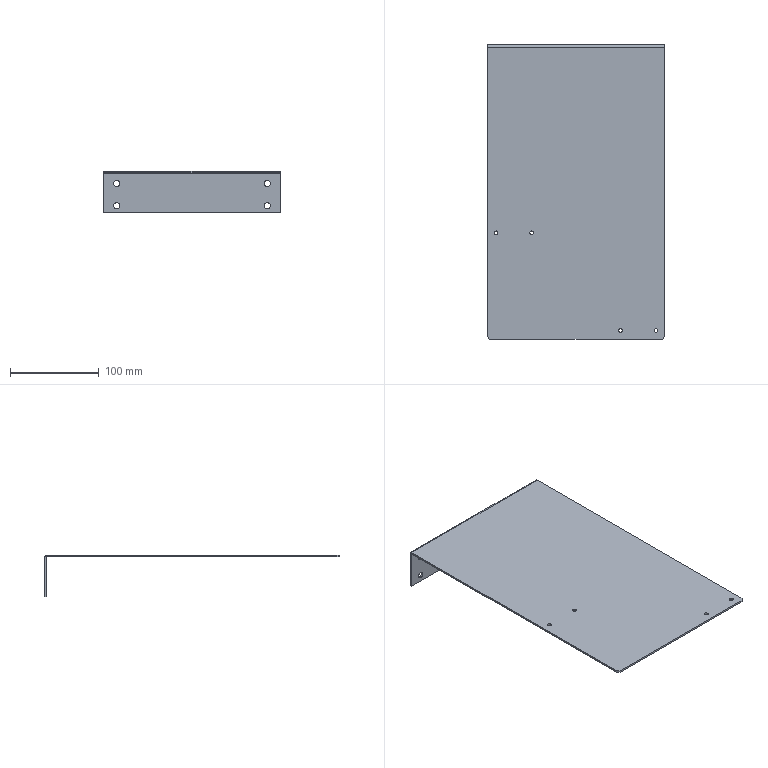Part | SolidWorks | features BaseBody 1 | 1 solid | 28 faces | box 200 x 332 x 47 mm | volume 150065 mm3 | cylinder 18 | plane 10 | commonest cylinder face diameters 4.2 x8 7 x8 1.473 x1 5.473 x1
STEP:
#1=CARTESIAN_POINT('',(85.,0.,-15.5));
#2=VERTEX_POINT('',#1);
#3=CARTESIAN_POINT('',(85.,0.,-8.5));
#4=VERTEX_POINT('',#3);
#5=CARTESIAN_POINT('',(85.,0.,-12.));
#6=DIRECTION('',(0.,1.,0.));
#7=DIRECTION('',(0.,0.,-1.));
#8=AXIS2_PLACEMENT_3D('',#5,#6,#7);
#9=CIRCLE('',#8,3.5);
#10=EDGE_CURVE('',#2,#4,#9,.T.);
#11=ORIENTED_EDGE('',*,*,#10,.F.);
#12=CARTESIAN_POINT('',(85.,2.,-15.5));
#13=VERTEX_POINT('',#12);
#14=CARTESIAN_POINT('',(85.,-330.001,-15.5));
#15=DIRECTION('',(0.,1.,0.));
#16=VECTOR('',#15,1000.);
#17=LINE('',#14,#16);
#18=EDGE_CURVE('',#2,#13,#17,.T.);
#19=ORIENTED_EDGE('',*,*,#18,.T.);
#20=CARTESIAN_POINT('',(85.,2.,-8.5));
#21=VERTEX_POINT('',#20);
#22=CARTESIAN_POINT('',(85.,2.,-12.));
#23=DIRECTION('',(0.,1.,0.));
#24=DIRECTION('',(0.,0.,1.));
#25=AXIS2_PLACEMENT_3D('',#22,#23,#24);
#26=CIRCLE('',#25,3.5);
#27=EDGE_CURVE('',#13,#21,#26,.T.);
#28=ORIENTED_EDGE('',*,*,#27,.T.);
#29=CARTESIAN_POINT('',(85.,-330.001,-8.5));
#30=DIRECTION('',(0.,1.,0.));
#31=VECTOR('',#30,1000.);
#32=LINE('',#29,#31);
#33=EDGE_CURVE('',#4,#21,#32,.T.);
#34=ORIENTED_EDGE('',*,*,#33,.F.);
#35=EDGE_LOOP('',(#11,#19,#28,#34));
#36=FACE_OUTER_BOUND('',#35,.T.);
#37=CARTESIAN_POINT('',(85.,-330.001,-12.));
#38=DIRECTION('',(0.,1.,0.));
#39=DIRECTION('',(0.,0.,1.));
#40=AXIS2_PLACEMENT_3D('',#37,#38,#39);
#41=CYLINDRICAL_SURFACE('',#40,3.5);
#42=ADVANCED_FACE('',(#36),#41,.F.);
#43=CARTESIAN_POINT('',(85.,0.,-40.5));
#44=VERTEX_POINT('',#43);
#45=CARTESIAN_POINT('',(85.,0.,-33.5));
#46=VERTEX_POINT('',#45);
#47=CARTESIAN_POINT('',(85.,0.,-37.));
#48=DIRECTION('',(0.,1.,0.));
#49=DIRECTION('',(0.,0.,-1.));
#50=AXIS2_PLACEMENT_3D('',#47,#48,#49);
#51=CIRCLE('',#50,3.5);
#52=EDGE_CURVE('',#44,#46,#51,.T.);
#53=ORIENTED_EDGE('',*,*,#52,.F.);
#54=CARTESIAN_POINT('',(85.,2.,-40.5));
#55=VERTEX_POINT('',#54);
#56=CARTESIAN_POINT('',(85.,-330.001,-40.5));
#57=DIRECTION('',(0.,1.,0.));
#58=VECTOR('',#57,1000.);
#59=LINE('',#56,#58);
#60=EDGE_CURVE('',#44,#55,#59,.T.);
#61=ORIENTED_EDGE('',*,*,#60,.T.);
#62=CARTESIAN_POINT('',(85.,2.,-33.5));
#63=VERTEX_POINT('',#62);
#64=CARTESIAN_POINT('',(85.,2.,-37.));
#65=DIRECTION('',(0.,1.,0.));
#66=DIRECTION('',(0.,0.,-1.));
#67=AXIS2_PLACEMENT_3D('',#64,#65,#66);
#68=CIRCLE('',#67,3.5);
#69=EDGE_CURVE('',#55,#63,#68,.T.);
#70=ORIENTED_EDGE('',*,*,#69,.T.);
#71=CARTESIAN_POINT('',(85.,-330.001,-33.5));
#72=DIRECTION('',(0.,1.,0.));
#73=VECTOR('',#72,1000.);
#74=LINE('',#71,#73);
#75=EDGE_CURVE('',#46,#63,#74,.T.);
#76=ORIENTED_EDGE('',*,*,#75,.F.);
#77=EDGE_LOOP('',(#53,#61,#70,#76));
#78=FACE_OUTER_BOUND('',#77,.T.);
#79=CARTESIAN_POINT('',(85.,-330.001,-37.));
#80=DIRECTION('',(0.,1.,0.));
#81=DIRECTION('',(0.,0.,1.));
#82=AXIS2_PLACEMENT_3D('',#79,#80,#81);
#83=CYLINDRICAL_SURFACE('',#82,3.5);
#84=ADVANCED_FACE('',(#78),#83,.F.);
#85=CARTESIAN_POINT('',(-85.,0.,-15.5));
#86=VERTEX_POINT('',#85);
#87=CARTESIAN_POINT('',(-85.,0.,-8.5));
#88=VERTEX_POINT('',#87);
#89=CARTESIAN_POINT('',(-85.,0.,-12.));
#90=DIRECTION('',(0.,1.,0.));
#91=DIRECTION('',(0.,0.,-1.));
#92=AXIS2_PLACEMENT_3D('',#89,#90,#91);
#93=CIRCLE('',#92,3.5);
#94=EDGE_CURVE('',#86,#88,#93,.T.);
#95=ORIENTED_EDGE('',*,*,#94,.F.);
#96=CARTESIAN_POINT('',(-85.,2.,-15.5));
#97=VERTEX_POINT('',#96);
#98=CARTESIAN_POINT('',(-85.,-330.001,-15.5));
#99=DIRECTION('',(0.,1.,0.));
#100=VECTOR('',#99,1000.);
#101=LINE('',#98,#100);
#102=EDGE_CURVE('',#86,#97,#101,.T.);
#103=ORIENTED_EDGE('',*,*,#102,.T.);
#104=CARTESIAN_POINT('',(-85.,2.,-8.5));
#105=VERTEX_POINT('',#104);
#106=CARTESIAN_POINT('',(-85.,2.,-12.));
#107=DIRECTION('',(0.,1.,0.));
#108=DIRECTION('',(0.,0.,-1.));
#109=AXIS2_PLACEMENT_3D('',#106,#107,#108);
#110=CIRCLE('',#109,3.5);
#111=EDGE_CURVE('',#97,#105,#110,.T.);
#112=ORIENTED_EDGE('',*,*,#111,.T.);
#113=CARTESIAN_POINT('',(-85.,-330.001,-8.5));
#114=DIRECTION('',(0.,1.,0.));
#115=VECTOR('',#114,1000.);
#116=LINE('',#113,#115);
#117=EDGE_CURVE('',#88,#105,#116,.T.);
#118=ORIENTED_EDGE('',*,*,#117,.F.);
#119=EDGE_LOOP('',(#95,#103,#112,#118));
#120=FACE_OUTER_BOUND('',#119,.T.);
#121=CARTESIAN_POINT('',(-85.,-330.001,-12.));
#122=DIRECTION('',(0.,1.,0.));
#123=DIRECTION('',(0.,0.,1.));
#124=AXIS2_PLACEMENT_3D('',#121,#122,#123);
#125=CYLINDRICAL_SURFACE('',#124,3.5);
#126=ADVANCED_FACE('',(#120),#125,.F.);
#127=CARTESIAN_POINT('',(-85.,0.,-40.5));
#128=VERTEX_POINT('',#127);
#129=CARTESIAN_POINT('',(-85.,0.,-33.5));
#130=VERTEX_POINT('',#129);
#131=CARTESIAN_POINT('',(-85.,0.,-37.));
#132=DIRECTION('',(0.,1.,0.));
#133=DIRECTION('',(0.,0.,-1.));
#134=AXIS2_PLACEMENT_3D('',#131,#132,#133);
#135=CIRCLE('',#134,3.5);
#136=EDGE_CURVE('',#128,#130,#135,.T.);
#137=ORIENTED_EDGE('',*,*,#136,.F.);
#138=CARTESIAN_POINT('',(-85.,2.,-40.5));
#139=VERTEX_POINT('',#138);
#140=CARTESIAN_POINT('',(-85.,-330.001,-40.5));
#141=DIRECTION('',(0.,1.,0.));
#142=VECTOR('',#141,1000.);
#143=LINE('',#140,#142);
#144=EDGE_CURVE('',#128,#139,#143,.T.);
#145=ORIENTED_EDGE('',*,*,#144,.T.);
#146=CARTESIAN_POINT('',(-85.,2.,-33.5));
#147=VERTEX_POINT('',#146);
#148=CARTESIAN_POINT('',(-85.,2.,-37.));
#149=DIRECTION('',(0.,1.,0.));
#150=DIRECTION('',(0.,0.,1.));
#151=AXIS2_PLACEMENT_3D('',#148,#149,#150);
#152=CIRCLE('',#151,3.5);
#153=EDGE_CURVE('',#139,#147,#152,.T.);
#154=ORIENTED_EDGE('',*,*,#153,.T.);
#155=CARTESIAN_POINT('',(-85.,-330.001,-33.5));
#156=DIRECTION('',(0.,1.,0.));
#157=VECTOR('',#156,1000.);
#158=LINE('',#155,#157);
#159=EDGE_CURVE('',#130,#147,#158,.T.);
#160=ORIENTED_EDGE('',*,*,#159,.F.);
#161=EDGE_LOOP('',(#137,#145,#154,#160));
#162=FACE_OUTER_BOUND('',#161,.T.);
#163=CARTESIAN_POINT('',(-85.,-330.001,-37.));
#164=DIRECTION('',(0.,1.,0.));
#165=DIRECTION('',(0.,0.,1.));
#166=AXIS2_PLACEMENT_3D('',#163,#164,#165);
#167=CYLINDRICAL_SURFACE('',#166,3.5);
#168=ADVANCED_FACE('',(#162),#167,.F.);
#169=CARTESIAN_POINT('',(90.,-322.1,2.));
#170=VERTEX_POINT('',#169);
#171=CARTESIAN_POINT('',(90.,-317.9,2.));
#172=VERTEX_POINT('',#171);
#173=CARTESIAN_POINT('',(90.,-320.,2.));
#174=DIRECTION('',(0.,0.,-1.));
#175=DIRECTION('',(0.,1.,0.));
#176=AXIS2_PLACEMENT_3D('',#173,#174,#175);
#177=CIRCLE('',#176,2.1);
#178=EDGE_CURVE('',#170,#172,#177,.T.);
#179=ORIENTED_EDGE('',*,*,#178,.F.);
#180=CARTESIAN_POINT('',(90.,-322.1,0.));
#181=VERTEX_POINT('',#180);
#182=CARTESIAN_POINT('',(90.,-322.1,0.));
#183=DIRECTION('',(0.,0.,-1.));
#184=VECTOR('',#183,1000.);
#185=LINE('',#182,#184);
#186=EDGE_CURVE('',#170,#181,#185,.T.);
#187=ORIENTED_EDGE('',*,*,#186,.T.);
#188=CARTESIAN_POINT('',(90.,-317.9,0.));
#189=VERTEX_POINT('',#188);
#190=CARTESIAN_POINT('',(90.,-320.,0.));
#191=DIRECTION('',(0.,0.,-1.));
#192=DIRECTION('',(0.,1.,0.));
#193=AXIS2_PLACEMENT_3D('',#190,#191,#192);
#194=CIRCLE('',#193,2.1);
#195=EDGE_CURVE('',#181,#189,#194,.T.);
#196=ORIENTED_EDGE('',*,*,#195,.T.);
#197=CARTESIAN_POINT('',(90.,-317.9,0.));
#198=DIRECTION('',(0.,0.,-1.));
#199=VECTOR('',#198,1000.);
#200=LINE('',#197,#199);
#201=EDGE_CURVE('',#172,#189,#200,.T.);
#202=ORIENTED_EDGE('',*,*,#201,.F.);
#203=EDGE_LOOP('',(#179,#187,#196,#202));
#204=FACE_OUTER_BOUND('',#203,.T.);
#205=CARTESIAN_POINT('',(90.,-320.,0.));
#206=DIRECTION('',(0.,0.,-1.));
#207=DIRECTION('',(0.,1.,0.));
#208=AXIS2_PLACEMENT_3D('',#205,#206,#207);
#209=CYLINDRICAL_SURFACE('',#208,2.1);
#210=ADVANCED_FACE('',(#204),#209,.F.);
#211=CARTESIAN_POINT('',(50.,-322.1,2.));
#212=VERTEX_POINT('',#211);
#213=CARTESIAN_POINT('',(50.,-317.9,2.));
#214=VERTEX_POINT('',#213);
#215=CARTESIAN_POINT('',(50.,-320.,2.));
#216=DIRECTION('',(0.,0.,-1.));
#217=DIRECTION('',(0.,1.,0.));
#218=AXIS2_PLACEMENT_3D('',#215,#216,#217);
#219=CIRCLE('',#218,2.1);
#220=EDGE_CURVE('',#212,#214,#219,.T.);
#221=ORIENTED_EDGE('',*,*,#220,.F.);
#222=CARTESIAN_POINT('',(50.,-322.1,0.));
#223=VERTEX_POINT('',#222);
#224=CARTESIAN_POINT('',(50.,-322.1,0.));
#225=DIRECTION('',(0.,0.,-1.));
#226=VECTOR('',#225,1000.);
#227=LINE('',#224,#226);
#228=EDGE_CURVE('',#212,#223,#227,.T.);
#229=ORIENTED_EDGE('',*,*,#228,.T.);
#230=CARTESIAN_POINT('',(50.,-317.9,0.));
#231=VERTEX_POINT('',#230);
#232=CARTESIAN_POINT('',(50.,-320.,0.));
#233=DIRECTION('',(0.,0.,-1.));
#234=DIRECTION('',(0.,1.,0.));
#235=AXIS2_PLACEMENT_3D('',#232,#233,#234);
#236=CIRCLE('',#235,2.1);
#237=EDGE_CURVE('',#223,#231,#236,.T.);
#238=ORIENTED_EDGE('',*,*,#237,.T.);
#239=CARTESIAN_POINT('',(50.,-317.9,0.));
#240=DIRECTION('',(0.,0.,-1.));
#241=VECTOR('',#240,1000.);
#242=LINE('',#239,#241);
#243=EDGE_CURVE('',#214,#231,#242,.T.);
#244=ORIENTED_EDGE('',*,*,#243,.F.);
#245=EDGE_LOOP('',(#221,#229,#238,#244));
#246=FACE_OUTER_BOUND('',#245,.T.);
#247=CARTESIAN_POINT('',(50.,-320.,0.));
#248=DIRECTION('',(0.,0.,-1.));
#249=DIRECTION('',(0.,1.,0.));
#250=AXIS2_PLACEMENT_3D('',#247,#248,#249);
#251=CYLINDRICAL_SURFACE('',#250,2.1);
#252=ADVANCED_FACE('',(#246),#251,.F.);
#253=CARTESIAN_POINT('',(-50.,-212.1,2.));
#254=VERTEX_POINT('',#253);
#255=CARTESIAN_POINT('',(-50.,-207.9,2.));
#256=VERTEX_POINT('',#255);
#257=CARTESIAN_POINT('',(-50.,-210.,2.));
#258=DIRECTION('',(0.,0.,-1.));
#259=DIRECTION('',(0.,1.,0.));
#260=AXIS2_PLACEMENT_3D('',#257,#258,#259);
#261=CIRCLE('',#260,2.1);
#262=EDGE_CURVE('',#254,#256,#261,.T.);
#263=ORIENTED_EDGE('',*,*,#262,.F.);
#264=CARTESIAN_POINT('',(-50.,-212.1,0.));
#265=VERTEX_POINT('',#264);
#266=CARTESIAN_POINT('',(-50.,-212.1,0.));
#267=DIRECTION('',(0.,0.,-1.));
#268=VECTOR('',#267,1000.);
#269=LINE('',#266,#268);
#270=EDGE_CURVE('',#254,#265,#269,.T.);
#271=ORIENTED_EDGE('',*,*,#270,.T.);
#272=CARTESIAN_POINT('',(-50.,-207.9,0.));
#273=VERTEX_POINT('',#272);
#274=CARTESIAN_POINT('',(-50.,-210.,0.));
#275=DIRECTION('',(0.,0.,-1.));
#276=DIRECTION('',(0.,1.,0.));
#277=AXIS2_PLACEMENT_3D('',#274,#275,#276);
#278=CIRCLE('',#277,2.1);
#279=EDGE_CURVE('',#265,#273,#278,.T.);
#280=ORIENTED_EDGE('',*,*,#279,.T.);
#281=CARTESIAN_POINT('',(-50.,-207.9,0.));
#282=DIRECTION('',(0.,0.,-1.));
#283=VECTOR('',#282,1000.);
#284=LINE('',#281,#283);
#285=EDGE_CURVE('',#256,#273,#284,.T.);
#286=ORIENTED_EDGE('',*,*,#285,.F.);
#287=EDGE_LOOP('',(#263,#271,#280,#286));
#288=FACE_OUTER_BOUND('',#287,.T.);
#289=CARTESIAN_POINT('',(-50.,-210.,0.));
#290=DIRECTION('',(0.,0.,-1.));
#291=DIRECTION('',(0.,1.,0.));
#292=AXIS2_PLACEMENT_3D('',#289,#290,#291);
#293=CYLINDRICAL_SURFACE('',#292,2.1);
#294=ADVANCED_FACE('',(#288),#293,.F.);
#295=CARTESIAN_POINT('',(-90.,-212.1,2.));
#296=VERTEX_POINT('',#295);
#297=CARTESIAN_POINT('',(-90.,-207.9,2.));
#298=VERTEX_POINT('',#297);
#299=CARTESIAN_POINT('',(-90.,-210.,2.));
#300=DIRECTION('',(0.,0.,-1.));
#301=DIRECTION('',(0.,1.,0.));
#302=AXIS2_PLACEMENT_3D('',#299,#300,#301);
#303=CIRCLE('',#302,2.1);
#304=EDGE_CURVE('',#296,#298,#303,.T.);
#305=ORIENTED_EDGE('',*,*,#304,.F.);
#306=CARTESIAN_POINT('',(-90.,-212.1,0.));
#307=VERTEX_POINT('',#306);
#308=CARTESIAN_POINT('',(-90.,-212.1,0.));
#309=DIRECTION('',(0.,0.,-1.));
#310=VECTOR('',#309,1000.);
#311=LINE('',#308,#310);
#312=EDGE_CURVE('',#296,#307,#311,.T.);
#313=ORIENTED_EDGE('',*,*,#312,.T.);
#314=CARTESIAN_POINT('',(-90.,-207.9,0.));
#315=VERTEX_POINT('',#314);
#316=CARTESIAN_POINT('',(-90.,-210.,0.));
#317=DIRECTION('',(0.,0.,-1.));
#318=DIRECTION('',(0.,1.,0.));
#319=AXIS2_PLACEMENT_3D('',#316,#317,#318);
#320=CIRCLE('',#319,2.1);
#321=EDGE_CURVE('',#307,#315,#320,.T.);
#322=ORIENTED_EDGE('',*,*,#321,.T.);
#323=CARTESIAN_POINT('',(-90.,-207.9,0.));
#324=DIRECTION('',(0.,0.,-1.));
#325=VECTOR('',#324,1000.);
#326=LINE('',#323,#325);
#327=EDGE_CURVE('',#298,#315,#326,.T.);
#328=ORIENTED_EDGE('',*,*,#327,.F.);
#329=EDGE_LOOP('',(#305,#313,#322,#328));
#330=FACE_OUTER_BOUND('',#329,.T.);
#331=CARTESIAN_POINT('',(-90.,-210.,0.));
#332=DIRECTION('',(0.,0.,-1.));
#333=DIRECTION('',(0.,1.,0.));
#334=AXIS2_PLACEMENT_3D('',#331,#332,#333);
#335=CYLINDRICAL_SURFACE('',#334,2.1);
#336=ADVANCED_FACE('',(#330),#335,.F.);
#337=CARTESIAN_POINT('',(100.,-327.,0.));
#338=VERTEX_POINT('',#337);
#339=CARTESIAN_POINT('',(97.,-330.,0.));
#340=VERTEX_POINT('',#339);
#341=CARTESIAN_POINT('',(263.5,-163.5,0.));
#342=DIRECTION('',(-0.7071,-0.7071,0.));
#343=VECTOR('',#342,1000.);
#344=LINE('',#341,#343);
#345=EDGE_CURVE('',#338,#340,#344,.T.);
#346=ORIENTED_EDGE('',*,*,#345,.F.);
#347=CARTESIAN_POINT('',(100.,-327.,2.));
#348=VERTEX_POINT('',#347);
#349=CARTESIAN_POINT('',(100.,-327.,-0.7366));
#350=DIRECTION('',(0.,0.,-1.));
#351=VECTOR('',#350,1000.);
#352=LINE('',#349,#351);
#353=EDGE_CURVE('',#348,#338,#352,.T.);
#354=ORIENTED_EDGE('',*,*,#353,.F.);
#355=CARTESIAN_POINT('',(97.,-330.,2.));
#356=VERTEX_POINT('',#355);
#357=CARTESIAN_POINT('',(97.,-330.,2.));
#358=DIRECTION('',(0.7071,0.7071,0.));
#359=VECTOR('',#358,1000.);
#360=LINE('',#357,#359);
#361=EDGE_CURVE('',#356,#348,#360,.T.);
#362=ORIENTED_EDGE('',*,*,#361,.F.);
#363=CARTESIAN_POINT('',(97.,-330.,0.));
#364=DIRECTION('',(0.,0.,1.));
#365=VECTOR('',#364,1000.);
#366=LINE('',#363,#365);
#367=EDGE_CURVE('',#340,#356,#366,.T.);
#368=ORIENTED_EDGE('',*,*,#367,.F.);
#369=EDGE_LOOP('',(#346,#354,#362,#368));
#370=FACE_OUTER_BOUND('',#369,.T.);
#371=CARTESIAN_POINT('',(97.,-330.,0.));
#372=DIRECTION('',(-0.7071,0.7071,0.));
#373=DIRECTION('',(0.,0.,1.));
#374=AXIS2_PLACEMENT_3D('',#371,#372,#373);
#375=PLANE('',#374);
#376=ADVANCED_FACE('',(#370),#375,.F.);
#377=CARTESIAN_POINT('',(-97.,-330.,0.));
#378=VERTEX_POINT('',#377);
#379=CARTESIAN_POINT('',(-100.,-327.,0.));
#380=VERTEX_POINT('',#379);
#381=CARTESIAN_POINT('',(-163.5,-263.5,0.));
#382=DIRECTION('',(-0.7071,0.7071,0.));
#383=VECTOR('',#382,1000.);
#384=LINE('',#381,#383);
#385=EDGE_CURVE('',#378,#380,#384,.T.);
#386=ORIENTED_EDGE('',*,*,#385,.F.);
#387=CARTESIAN_POINT('',(-97.,-330.,2.));
#388=VERTEX_POINT('',#387);
#389=CARTESIAN_POINT('',(-97.,-330.,0.));
#390=DIRECTION('',(0.,0.,-1.));
#391=VECTOR('',#390,1000.);
#392=LINE('',#389,#391);
#393=EDGE_CURVE('',#388,#378,#392,.T.);
#394=ORIENTED_EDGE('',*,*,#393,.F.);
#395=CARTESIAN_POINT('',(-100.,-327.,2.));
#396=VERTEX_POINT('',#395);
#397=CARTESIAN_POINT('',(-100.,-327.,2.));
#398=DIRECTION('',(0.7071,-0.7071,0.));
#399=VECTOR('',#398,1000.);
#400=LINE('',#397,#399);
#401=EDGE_CURVE('',#396,#388,#400,.T.);
#402=ORIENTED_EDGE('',*,*,#401,.F.);
#403=CARTESIAN_POINT('',(-100.,-327.,-0.7366));
#404=DIRECTION('',(0.,0.,1.));
#405=VECTOR('',#404,1000.);
#406=LINE('',#403,#405);
#407=EDGE_CURVE('',#380,#396,#406,.T.);
#408=ORIENTED_EDGE('',*,*,#407,.F.);
#409=EDGE_LOOP('',(#386,#394,#402,#408));
#410=FACE_OUTER_BOUND('',#409,.T.);
#411=CARTESIAN_POINT('',(-100.,-327.,-0.7366));
#412=DIRECTION('',(0.7071,0.7071,0.));
#413=DIRECTION('',(0.,0.,-1.));
#414=AXIS2_PLACEMENT_3D('',#411,#412,#413);
#415=PLANE('',#414);
#416=ADVANCED_FACE('',(#410),#415,.F.);
#417=CARTESIAN_POINT('',(-100.,2.,-0.7366));
#418=VERTEX_POINT('',#417);
#419=CARTESIAN_POINT('',(-100.,-0.7366,2.));
#420=VERTEX_POINT('',#419);
#421=CARTESIAN_POINT('',(-100.,-0.7366,-0.7366));
#422=DIRECTION('',(1.,0.,0.));
#423=DIRECTION('',(0.,0.,-1.));
#424=AXIS2_PLACEMENT_3D('',#421,#422,#423);
#425=CIRCLE('',#424,2.737);
#426=EDGE_CURVE('',#418,#420,#425,.T.);
#427=ORIENTED_EDGE('',*,*,#426,.T.);
#428=CARTESIAN_POINT('',(100.,-0.7366,2.));
#429=VERTEX_POINT('',#428);
#430=CARTESIAN_POINT('',(100.,-0.7366,2.));
#431=DIRECTION('',(-1.,0.,0.));
#432=VECTOR('',#431,1000.);
#433=LINE('',#430,#432);
#434=EDGE_CURVE('',#429,#420,#433,.T.);
#435=ORIENTED_EDGE('',*,*,#434,.F.);
#436=CARTESIAN_POINT('',(100.,2.,-0.7366));
#437=VERTEX_POINT('',#436);
#438=CARTESIAN_POINT('',(100.,-0.7366,-0.7366));
#439=DIRECTION('',(1.,0.,0.));
#440=DIRECTION('',(0.,0.,-1.));
#441=AXIS2_PLACEMENT_3D('',#438,#439,#440);
#442=CIRCLE('',#441,2.737);
#443=EDGE_CURVE('',#437,#429,#442,.T.);
#444=ORIENTED_EDGE('',*,*,#443,.F.);
#445=CARTESIAN_POINT('',(100.,2.,-0.7366));
#446=DIRECTION('',(-1.,0.,0.));
#447=VECTOR('',#446,1000.);
#448=LINE('',#445,#447);
#449=EDGE_CURVE('',#437,#418,#448,.T.);
#450=ORIENTED_EDGE('',*,*,#449,.T.);
#451=EDGE_LOOP('',(#427,#435,#444,#450));
#452=FACE_OUTER_BOUND('',#451,.T.);
#453=CARTESIAN_POINT('',(100.,-0.7366,-0.7366));
#454=DIRECTION('',(-1.,0.,0.));
#455=DIRECTION('',(0.,0.,1.));
#456=AXIS2_PLACEMENT_3D('',#453,#454,#455);
#457=CYLINDRICAL_SURFACE('',#456,2.737);
#458=ADVANCED_FACE('',(#452),#457,.T.);
#459=CARTESIAN_POINT('',(-85.,2.,-37.));
#460=DIRECTION('',(0.,1.,0.));
#461=DIRECTION('',(0.,0.,1.));
#462=AXIS2_PLACEMENT_3D('',#459,#460,#461);
#463=CIRCLE('',#462,3.5);
#464=EDGE_CURVE('',#147,#139,#463,.T.);
#465=ORIENTED_EDGE('',*,*,#464,.F.);
#466=ORIENTED_EDGE('',*,*,#153,.F.);
#467=EDGE_LOOP('',(#465,#466));
#468=FACE_BOUND('',#467,.T.);
#469=CARTESIAN_POINT('',(-85.,2.,-12.));
#470=DIRECTION('',(0.,1.,0.));
#471=DIRECTION('',(0.,0.,-1.));
#472=AXIS2_PLACEMENT_3D('',#469,#470,#471);
#473=CIRCLE('',#472,3.5);
#474=EDGE_CURVE('',#105,#97,#473,.T.);
#475=ORIENTED_EDGE('',*,*,#474,.F.);
#476=ORIENTED_EDGE('',*,*,#111,.F.);
#477=EDGE_LOOP('',(#475,#476));
#478=FACE_BOUND('',#477,.T.);
#479=CARTESIAN_POINT('',(85.,2.,-37.));
#480=DIRECTION('',(0.,1.,0.));
#481=DIRECTION('',(0.,0.,-1.));
#482=AXIS2_PLACEMENT_3D('',#479,#480,#481);
#483=CIRCLE('',#482,3.5);
#484=EDGE_CURVE('',#63,#55,#483,.T.);
#485=ORIENTED_EDGE('',*,*,#484,.F.);
#486=ORIENTED_EDGE('',*,*,#69,.F.);
#487=EDGE_LOOP('',(#485,#486));
#488=FACE_BOUND('',#487,.T.);
#489=CARTESIAN_POINT('',(85.,2.,-12.));
#490=DIRECTION('',(0.,1.,0.));
#491=DIRECTION('',(0.,0.,1.));
#492=AXIS2_PLACEMENT_3D('',#489,#490,#491);
#493=CIRCLE('',#492,3.5);
#494=EDGE_CURVE('',#21,#13,#493,.T.);
#495=ORIENTED_EDGE('',*,*,#494,.F.);
#496=ORIENTED_EDGE('',*,*,#27,.F.);
#497=EDGE_LOOP('',(#495,#496));
#498=FACE_BOUND('',#497,.T.);
#499=CARTESIAN_POINT('',(-100.,2.,-45.));
#500=VERTEX_POINT('',#499);
#501=CARTESIAN_POINT('',(-100.,2.,-45.));
#502=DIRECTION('',(0.,0.,1.));
#503=VECTOR('',#502,1000.);
#504=LINE('',#501,#503);
#505=EDGE_CURVE('',#500,#418,#504,.T.);
#506=ORIENTED_EDGE('',*,*,#505,.T.);
#507=ORIENTED_EDGE('',*,*,#449,.F.);
#508=CARTESIAN_POINT('',(100.,2.,-45.));
#509=VERTEX_POINT('',#508);
#510=CARTESIAN_POINT('',(100.,2.,-45.));
#511=DIRECTION('',(0.,0.,1.));
#512=VECTOR('',#511,1000.);
#513=LINE('',#510,#512);
#514=EDGE_CURVE('',#509,#437,#513,.T.);
#515=ORIENTED_EDGE('',*,*,#514,.F.);
#516=CARTESIAN_POINT('',(100.,2.,-45.));
#517=DIRECTION('',(-1.,0.,0.));
#518=VECTOR('',#517,1000.);
#519=LINE('',#516,#518);
#520=EDGE_CURVE('',#509,#500,#519,.T.);
#521=ORIENTED_EDGE('',*,*,#520,.T.);
#522=EDGE_LOOP('',(#506,#507,#515,#521));
#523=FACE_OUTER_BOUND('',#522,.T.);
#524=CARTESIAN_POINT('',(100.,2.,-45.));
#525=DIRECTION('',(0.,-1.,0.));
#526=DIRECTION('',(0.,0.,-1.));
#527=AXIS2_PLACEMENT_3D('',#524,#525,#526);
#528=PLANE('',#527);
#529=ADVANCED_FACE('',(#468,#478,#488,#498,#523),#528,.F.);
#530=CARTESIAN_POINT('',(-100.,0.,-45.));
#531=VERTEX_POINT('',#530);
#532=CARTESIAN_POINT('',(-100.,2.,-45.));
#533=DIRECTION('',(0.,-1.,0.));
#534=VECTOR('',#533,1000.);
#535=LINE('',#532,#534);
#536=EDGE_CURVE('',#500,#531,#535,.T.);
#537=ORIENTED_EDGE('',*,*,#536,.F.);
#538=ORIENTED_EDGE('',*,*,#520,.F.);
#539=CARTESIAN_POINT('',(100.,0.,-45.));
#540=VERTEX_POINT('',#539);
#541=CARTESIAN_POINT('',(100.,2.,-45.));
#542=DIRECTION('',(0.,-1.,0.));
#543=VECTOR('',#542,1000.);
#544=LINE('',#541,#543);
#545=EDGE_CURVE('',#509,#540,#544,.T.);
#546=ORIENTED_EDGE('',*,*,#545,.T.);
#547=CARTESIAN_POINT('',(100.,0.,-45.));
#548=DIRECTION('',(-1.,0.,0.));
#549=VECTOR('',#548,1000.);
#550=LINE('',#547,#549);
#551=EDGE_CURVE('',#540,#531,#550,.T.);
#552=ORIENTED_EDGE('',*,*,#551,.T.);
#553=EDGE_LOOP('',(#537,#538,#546,#552));
#554=FACE_OUTER_BOUND('',#553,.T.);
#555=CARTESIAN_POINT('',(100.,2.,-45.));
#556=DIRECTION('',(0.,0.,-1.));
#557=DIRECTION('',(0.,-1.,0.));
#558=AXIS2_PLACEMENT_3D('',#555,#556,#557);
#559=PLANE('',#558);
#560=ADVANCED_FACE('',(#554),#559,.T.);
#561=CARTESIAN_POINT('',(-85.,0.,-37.));
#562=DIRECTION('',(0.,1.,0.));
#563=DIRECTION('',(0.,0.,-1.));
#564=AXIS2_PLACEMENT_3D('',#561,#562,#563);
#565=CIRCLE('',#564,3.5);
#566=EDGE_CURVE('',#130,#128,#565,.T.);
#567=ORIENTED_EDGE('',*,*,#566,.T.);
#568=ORIENTED_EDGE('',*,*,#136,.T.);
#569=EDGE_LOOP('',(#567,#568));
#570=FACE_BOUND('',#569,.T.);
#571=CARTESIAN_POINT('',(-85.,0.,-12.));
#572=DIRECTION('',(0.,1.,0.));
#573=DIRECTION('',(0.,0.,-1.));
#574=AXIS2_PLACEMENT_3D('',#571,#572,#573);
#575=CIRCLE('',#574,3.5);
#576=EDGE_CURVE('',#88,#86,#575,.T.);
#577=ORIENTED_EDGE('',*,*,#576,.T.);
#578=ORIENTED_EDGE('',*,*,#94,.T.);
#579=EDGE_LOOP('',(#577,#578));
#580=FACE_BOUND('',#579,.T.);
#581=CARTESIAN_POINT('',(85.,0.,-37.));
#582=DIRECTION('',(0.,1.,0.));
#583=DIRECTION('',(0.,0.,-1.));
#584=AXIS2_PLACEMENT_3D('',#581,#582,#583);
#585=CIRCLE('',#584,3.5);
#586=EDGE_CURVE('',#46,#44,#585,.T.);
#587=ORIENTED_EDGE('',*,*,#586,.T.);
#588=ORIENTED_EDGE('',*,*,#52,.T.);
#589=EDGE_LOOP('',(#587,#588));
#590=FACE_BOUND('',#589,.T.);
#591=CARTESIAN_POINT('',(85.,0.,-12.));
#592=DIRECTION('',(0.,1.,0.));
#593=DIRECTION('',(0.,0.,-1.));
#594=AXIS2_PLACEMENT_3D('',#591,#592,#593);
#595=CIRCLE('',#594,3.5);
#596=EDGE_CURVE('',#4,#2,#595,.T.);
#597=ORIENTED_EDGE('',*,*,#596,.T.);
#598=ORIENTED_EDGE('',*,*,#10,.T.);
#599=EDGE_LOOP('',(#597,#598));
#600=FACE_BOUND('',#599,.T.);
#601=CARTESIAN_POINT('',(-100.,0.,-0.7366));
#602=VERTEX_POINT('',#601);
#603=CARTESIAN_POINT('',(-100.,0.,-45.));
#604=DIRECTION('',(0.,0.,1.));
#605=VECTOR('',#604,1000.);
#606=LINE('',#603,#605);
#607=EDGE_CURVE('',#531,#602,#606,.T.);
#608=ORIENTED_EDGE('',*,*,#607,.F.);
#609=ORIENTED_EDGE('',*,*,#551,.F.);
#610=CARTESIAN_POINT('',(100.,0.,-0.7366));
#611=VERTEX_POINT('',#610);
#612=CARTESIAN_POINT('',(100.,0.,-45.));
#613=DIRECTION('',(0.,0.,1.));
#614=VECTOR('',#613,1000.);
#615=LINE('',#612,#614);
#616=EDGE_CURVE('',#540,#611,#615,.T.);
#617=ORIENTED_EDGE('',*,*,#616,.T.);
#618=CARTESIAN_POINT('',(100.,0.,-0.7366));
#619=DIRECTION('',(-1.,0.,0.));
#620=VECTOR('',#619,1000.);
#621=LINE('',#618,#620);
#622=EDGE_CURVE('',#611,#602,#621,.T.);
#623=ORIENTED_EDGE('',*,*,#622,.T.);
#624=EDGE_LOOP('',(#608,#609,#617,#623));
#625=FACE_OUTER_BOUND('',#624,.T.);
#626=CARTESIAN_POINT('',(100.,0.,-45.));
#627=DIRECTION('',(0.,-1.,0.));
#628=DIRECTION('',(0.,0.,-1.));
#629=AXIS2_PLACEMENT_3D('',#626,#627,#628);
#630=PLANE('',#629);
#631=ADVANCED_FACE('',(#570,#580,#590,#600,#625),#630,.T.);
#632=CARTESIAN_POINT('',(-100.,-0.7366,0.));
#633=VERTEX_POINT('',#632);
#634=CARTESIAN_POINT('',(-100.,-0.7366,-0.7366));
#635=DIRECTION('',(1.,0.,0.));
#636=DIRECTION('',(0.,0.,1.));
#637=AXIS2_PLACEMENT_3D('',#634,#635,#636);
#638=CIRCLE('',#637,0.7366);
#639=EDGE_CURVE('',#602,#633,#638,.T.);
#640=ORIENTED_EDGE('',*,*,#639,.F.);
#641=ORIENTED_EDGE('',*,*,#622,.F.);
#642=CARTESIAN_POINT('',(100.,-0.7366,0.));
#643=VERTEX_POINT('',#642);
#644=CARTESIAN_POINT('',(100.,-0.7366,-0.7366));
#645=DIRECTION('',(1.,0.,0.));
#646=DIRECTION('',(0.,0.,1.));
#647=AXIS2_PLACEMENT_3D('',#644,#645,#646);
#648=CIRCLE('',#647,0.7366);
#649=EDGE_CURVE('',#611,#643,#648,.T.);
#650=ORIENTED_EDGE('',*,*,#649,.T.);
#651=CARTESIAN_POINT('',(100.,-0.7366,0.));
#652=DIRECTION('',(-1.,0.,0.));
#653=VECTOR('',#652,1000.);
#654=LINE('',#651,#653);
#655=EDGE_CURVE('',#643,#633,#654,.T.);
#656=ORIENTED_EDGE('',*,*,#655,.T.);
#657=EDGE_LOOP('',(#640,#641,#650,#656));
#658=FACE_OUTER_BOUND('',#657,.T.);
#659=CARTESIAN_POINT('',(100.,-0.7366,-0.7366));
#660=DIRECTION('',(-1.,0.,0.));
#661=DIRECTION('',(0.,0.,1.));
#662=AXIS2_PLACEMENT_3D('',#659,#660,#661);
#663=CYLINDRICAL_SURFACE('',#662,0.7366);
#664=ADVANCED_FACE('',(#658),#663,.F.);
#665=CARTESIAN_POINT('',(-90.,-210.,0.));
#666=DIRECTION('',(0.,0.,-1.));
#667=DIRECTION('',(0.,1.,0.));
#668=AXIS2_PLACEMENT_3D('',#665,#666,#667);
#669=CIRCLE('',#668,2.1);
#670=EDGE_CURVE('',#315,#307,#669,.T.);
#671=ORIENTED_EDGE('',*,*,#670,.F.);
#672=ORIENTED_EDGE('',*,*,#321,.F.);
#673=EDGE_LOOP('',(#671,#672));
#674=FACE_BOUND('',#673,.T.);
#675=CARTESIAN_POINT('',(-50.,-210.,0.));
#676=DIRECTION('',(0.,0.,-1.));
#677=DIRECTION('',(0.,1.,0.));
#678=AXIS2_PLACEMENT_3D('',#675,#676,#677);
#679=CIRCLE('',#678,2.1);
#680=EDGE_CURVE('',#273,#265,#679,.T.);
#681=ORIENTED_EDGE('',*,*,#680,.F.);
#682=ORIENTED_EDGE('',*,*,#279,.F.);
#683=EDGE_LOOP('',(#681,#682));
#684=FACE_BOUND('',#683,.T.);
#685=CARTESIAN_POINT('',(50.,-320.,0.));
#686=DIRECTION('',(0.,0.,-1.));
#687=DIRECTION('',(0.,1.,0.));
#688=AXIS2_PLACEMENT_3D('',#685,#686,#687);
#689=CIRCLE('',#688,2.1);
#690=EDGE_CURVE('',#231,#223,#689,.T.);
#691=ORIENTED_EDGE('',*,*,#690,.F.);
#692=ORIENTED_EDGE('',*,*,#237,.F.);
#693=EDGE_LOOP('',(#691,#692));
#694=FACE_BOUND('',#693,.T.);
#695=CARTESIAN_POINT('',(90.,-320.,0.));
#696=DIRECTION('',(0.,0.,-1.));
#697=DIRECTION('',(0.,1.,0.));
#698=AXIS2_PLACEMENT_3D('',#695,#696,#697);
#699=CIRCLE('',#698,2.1);
#700=EDGE_CURVE('',#189,#181,#699,.T.);
#701=ORIENTED_EDGE('',*,*,#700,.F.);
#702=ORIENTED_EDGE('',*,*,#195,.F.);
#703=EDGE_LOOP('',(#701,#702));
#704=FACE_BOUND('',#703,.T.);
#705=CARTESIAN_POINT('',(100.,-330.,0.));
#706=DIRECTION('',(-1.,0.,0.));
#707=VECTOR('',#706,1000.);
#708=LINE('',#705,#707);
#709=EDGE_CURVE('',#340,#378,#708,.T.);
#710=ORIENTED_EDGE('',*,*,#709,.T.);
#711=ORIENTED_EDGE('',*,*,#385,.T.);
#712=CARTESIAN_POINT('',(-100.,0.,0.));
#713=DIRECTION('',(0.,-1.,0.));
#714=VECTOR('',#713,1000.);
#715=LINE('',#712,#714);
#716=EDGE_CURVE('',#633,#380,#715,.T.);
#717=ORIENTED_EDGE('',*,*,#716,.F.);
#718=ORIENTED_EDGE('',*,*,#655,.F.);
#719=CARTESIAN_POINT('',(100.,0.,0.));
#720=DIRECTION('',(0.,-1.,0.));
#721=VECTOR('',#720,1000.);
#722=LINE('',#719,#721);
#723=EDGE_CURVE('',#643,#338,#722,.T.);
#724=ORIENTED_EDGE('',*,*,#723,.T.);
#725=ORIENTED_EDGE('',*,*,#345,.T.);
#726=EDGE_LOOP('',(#710,#711,#717,#718,#724,#725));
#727=FACE_OUTER_BOUND('',#726,.T.);
#728=CARTESIAN_POINT('',(100.,0.,0.));
#729=DIRECTION('',(0.,0.,-1.));
#730=DIRECTION('',(-1.,0.,0.));
#731=AXIS2_PLACEMENT_3D('',#728,#729,#730);
#732=PLANE('',#731);
#733=ADVANCED_FACE('',(#674,#684,#694,#704,#727),#732,.T.);
#734=CARTESIAN_POINT('',(100.,-330.,2.));
#735=DIRECTION('',(-1.,0.,0.));
#736=VECTOR('',#735,1000.);
#737=LINE('',#734,#736);
#738=EDGE_CURVE('',#356,#388,#737,.T.);
#739=ORIENTED_EDGE('',*,*,#738,.T.);
#740=ORIENTED_EDGE('',*,*,#393,.T.);
#741=ORIENTED_EDGE('',*,*,#709,.F.);
#742=ORIENTED_EDGE('',*,*,#367,.T.);
#743=EDGE_LOOP('',(#739,#740,#741,#742));
#744=FACE_OUTER_BOUND('',#743,.T.);
#745=CARTESIAN_POINT('',(100.,-330.,0.));
#746=DIRECTION('',(0.,-1.,0.));
#747=DIRECTION('',(0.,0.,-1.));
#748=AXIS2_PLACEMENT_3D('',#745,#746,#747);
#749=PLANE('',#748);
#750=ADVANCED_FACE('',(#744),#749,.T.);
#751=CARTESIAN_POINT('',(-90.,-210.,2.));
#752=DIRECTION('',(0.,0.,-1.));
#753=DIRECTION('',(0.,1.,0.));
#754=AXIS2_PLACEMENT_3D('',#751,#752,#753);
#755=CIRCLE('',#754,2.1);
#756=EDGE_CURVE('',#298,#296,#755,.T.);
#757=ORIENTED_EDGE('',*,*,#756,.T.);
#758=ORIENTED_EDGE('',*,*,#304,.T.);
#759=EDGE_LOOP('',(#757,#758));
#760=FACE_BOUND('',#759,.T.);
#761=CARTESIAN_POINT('',(-50.,-210.,2.));
#762=DIRECTION('',(0.,0.,-1.));
#763=DIRECTION('',(0.,1.,0.));
#764=AXIS2_PLACEMENT_3D('',#761,#762,#763);
#765=CIRCLE('',#764,2.1);
#766=EDGE_CURVE('',#256,#254,#765,.T.);
#767=ORIENTED_EDGE('',*,*,#766,.T.);
#768=ORIENTED_EDGE('',*,*,#262,.T.);
#769=EDGE_LOOP('',(#767,#768));
#770=FACE_BOUND('',#769,.T.);
#771=CARTESIAN_POINT('',(50.,-320.,2.));
#772=DIRECTION('',(0.,0.,-1.));
#773=DIRECTION('',(0.,1.,0.));
#774=AXIS2_PLACEMENT_3D('',#771,#772,#773);
#775=CIRCLE('',#774,2.1);
#776=EDGE_CURVE('',#214,#212,#775,.T.);
#777=ORIENTED_EDGE('',*,*,#776,.T.);
#778=ORIENTED_EDGE('',*,*,#220,.T.);
#779=EDGE_LOOP('',(#777,#778));
#780=FACE_BOUND('',#779,.T.);
#781=CARTESIAN_POINT('',(90.,-320.,2.));
#782=DIRECTION('',(0.,0.,-1.));
#783=DIRECTION('',(0.,1.,0.));
#784=AXIS2_PLACEMENT_3D('',#781,#782,#783);
#785=CIRCLE('',#784,2.1);
#786=EDGE_CURVE('',#172,#170,#785,.T.);
#787=ORIENTED_EDGE('',*,*,#786,.T.);
#788=ORIENTED_EDGE('',*,*,#178,.T.);
#789=EDGE_LOOP('',(#787,#788));
#790=FACE_BOUND('',#789,.T.);
#791=CARTESIAN_POINT('',(-100.,0.,2.));
#792=DIRECTION('',(0.,-1.,0.));
#793=VECTOR('',#792,1000.);
#794=LINE('',#791,#793);
#795=EDGE_CURVE('',#420,#396,#794,.T.);
#796=ORIENTED_EDGE('',*,*,#795,.T.);
#797=ORIENTED_EDGE('',*,*,#401,.T.);
#798=ORIENTED_EDGE('',*,*,#738,.F.);
#799=ORIENTED_EDGE('',*,*,#361,.T.);
#800=CARTESIAN_POINT('',(100.,0.,2.));
#801=DIRECTION('',(0.,-1.,0.));
#802=VECTOR('',#801,1000.);
#803=LINE('',#800,#802);
#804=EDGE_CURVE('',#429,#348,#803,.T.);
#805=ORIENTED_EDGE('',*,*,#804,.F.);
#806=ORIENTED_EDGE('',*,*,#434,.T.);
#807=EDGE_LOOP('',(#796,#797,#798,#799,#805,#806));
#808=FACE_OUTER_BOUND('',#807,.T.);
#809=CARTESIAN_POINT('',(100.,0.,2.));
#810=DIRECTION('',(0.,0.,-1.));
#811=DIRECTION('',(-1.,0.,0.));
#812=AXIS2_PLACEMENT_3D('',#809,#810,#811);
#813=PLANE('',#812);
#814=ADVANCED_FACE('',(#760,#770,#780,#790,#808),#813,.F.);
#815=ORIENTED_EDGE('',*,*,#426,.F.);
#816=ORIENTED_EDGE('',*,*,#505,.F.);
#817=ORIENTED_EDGE('',*,*,#536,.T.);
#818=ORIENTED_EDGE('',*,*,#607,.T.);
#819=ORIENTED_EDGE('',*,*,#639,.T.);
#820=ORIENTED_EDGE('',*,*,#716,.T.);
#821=ORIENTED_EDGE('',*,*,#407,.T.);
#822=ORIENTED_EDGE('',*,*,#795,.F.);
#823=EDGE_LOOP('',(#815,#816,#817,#818,#819,#820,#821,#822));
#824=FACE_OUTER_BOUND('',#823,.T.);
#825=CARTESIAN_POINT('',(-100.,0.,-0.7366));
#826=DIRECTION('',(-1.,0.,0.));
#827=DIRECTION('',(0.,0.,1.));
#828=AXIS2_PLACEMENT_3D('',#825,#826,#827);
#829=PLANE('',#828);
#830=ADVANCED_FACE('',(#824),#829,.T.);
#831=ORIENTED_EDGE('',*,*,#443,.T.);
#832=ORIENTED_EDGE('',*,*,#804,.T.);
#833=ORIENTED_EDGE('',*,*,#353,.T.);
#834=ORIENTED_EDGE('',*,*,#723,.F.);
#835=ORIENTED_EDGE('',*,*,#649,.F.);
#836=ORIENTED_EDGE('',*,*,#616,.F.);
#837=ORIENTED_EDGE('',*,*,#545,.F.);
#838=ORIENTED_EDGE('',*,*,#514,.T.);
#839=EDGE_LOOP('',(#831,#832,#833,#834,#835,#836,#837,#838));
#840=FACE_OUTER_BOUND('',#839,.T.);
#841=CARTESIAN_POINT('',(100.,-0.7366,0.));
#842=DIRECTION('',(1.,0.,0.));
#843=DIRECTION('',(0.,1.,0.));
#844=AXIS2_PLACEMENT_3D('',#841,#842,#843);
#845=PLANE('',#844);
#846=ADVANCED_FACE('',(#840),#845,.T.);
#847=ORIENTED_EDGE('',*,*,#312,.F.);
#848=ORIENTED_EDGE('',*,*,#756,.F.);
#849=ORIENTED_EDGE('',*,*,#327,.T.);
#850=ORIENTED_EDGE('',*,*,#670,.T.);
#851=EDGE_LOOP('',(#847,#848,#849,#850));
#852=FACE_OUTER_BOUND('',#851,.T.);
#853=CARTESIAN_POINT('',(-90.,-210.,0.));
#854=DIRECTION('',(0.,0.,-1.));
#855=DIRECTION('',(0.,1.,0.));
#856=AXIS2_PLACEMENT_3D('',#853,#854,#855);
#857=CYLINDRICAL_SURFACE('',#856,2.1);
#858=ADVANCED_FACE('',(#852),#857,.F.);
#859=ORIENTED_EDGE('',*,*,#270,.F.);
#860=ORIENTED_EDGE('',*,*,#766,.F.);
#861=ORIENTED_EDGE('',*,*,#285,.T.);
#862=ORIENTED_EDGE('',*,*,#680,.T.);
#863=EDGE_LOOP('',(#859,#860,#861,#862));
#864=FACE_OUTER_BOUND('',#863,.T.);
#865=CARTESIAN_POINT('',(-50.,-210.,0.));
#866=DIRECTION('',(0.,0.,-1.));
#867=DIRECTION('',(0.,1.,0.));
#868=AXIS2_PLACEMENT_3D('',#865,#866,#867);
#869=CYLINDRICAL_SURFACE('',#868,2.1);
#870=ADVANCED_FACE('',(#864),#869,.F.);
#871=ORIENTED_EDGE('',*,*,#228,.F.);
#872=ORIENTED_EDGE('',*,*,#776,.F.);
#873=ORIENTED_EDGE('',*,*,#243,.T.);
#874=ORIENTED_EDGE('',*,*,#690,.T.);
#875=EDGE_LOOP('',(#871,#872,#873,#874));
#876=FACE_OUTER_BOUND('',#875,.T.);
#877=CARTESIAN_POINT('',(50.,-320.,0.));
#878=DIRECTION('',(0.,0.,-1.));
#879=DIRECTION('',(0.,1.,0.));
#880=AXIS2_PLACEMENT_3D('',#877,#878,#879);
#881=CYLINDRICAL_SURFACE('',#880,2.1);
#882=ADVANCED_FACE('',(#876),#881,.F.);
#883=ORIENTED_EDGE('',*,*,#186,.F.);
#884=ORIENTED_EDGE('',*,*,#786,.F.);
#885=ORIENTED_EDGE('',*,*,#201,.T.);
#886=ORIENTED_EDGE('',*,*,#700,.T.);
#887=EDGE_LOOP('',(#883,#884,#885,#886));
#888=FACE_OUTER_BOUND('',#887,.T.);
#889=CARTESIAN_POINT('',(90.,-320.,0.));
#890=DIRECTION('',(0.,0.,-1.));
#891=DIRECTION('',(0.,1.,0.));
#892=AXIS2_PLACEMENT_3D('',#889,#890,#891);
#893=CYLINDRICAL_SURFACE('',#892,2.1);
#894=ADVANCED_FACE('',(#888),#893,.F.);
#895=ORIENTED_EDGE('',*,*,#144,.F.);
#896=ORIENTED_EDGE('',*,*,#566,.F.);
#897=ORIENTED_EDGE('',*,*,#159,.T.);
#898=ORIENTED_EDGE('',*,*,#464,.T.);
#899=EDGE_LOOP('',(#895,#896,#897,#898));
#900=FACE_OUTER_BOUND('',#899,.T.);
#901=CARTESIAN_POINT('',(-85.,-330.001,-37.));
#902=DIRECTION('',(0.,1.,0.));
#903=DIRECTION('',(0.,0.,1.));
#904=AXIS2_PLACEMENT_3D('',#901,#902,#903);
#905=CYLINDRICAL_SURFACE('',#904,3.5);
#906=ADVANCED_FACE('',(#900),#905,.F.);
#907=ORIENTED_EDGE('',*,*,#102,.F.);
#908=ORIENTED_EDGE('',*,*,#576,.F.);
#909=ORIENTED_EDGE('',*,*,#117,.T.);
#910=ORIENTED_EDGE('',*,*,#474,.T.);
#911=EDGE_LOOP('',(#907,#908,#909,#910));
#912=FACE_OUTER_BOUND('',#911,.T.);
#913=CARTESIAN_POINT('',(-85.,-330.001,-12.));
#914=DIRECTION('',(0.,1.,0.));
#915=DIRECTION('',(0.,0.,1.));
#916=AXIS2_PLACEMENT_3D('',#913,#914,#915);
#917=CYLINDRICAL_SURFACE('',#916,3.5);
#918=ADVANCED_FACE('',(#912),#917,.F.);
#919=ORIENTED_EDGE('',*,*,#60,.F.);
#920=ORIENTED_EDGE('',*,*,#586,.F.);
#921=ORIENTED_EDGE('',*,*,#75,.T.);
#922=ORIENTED_EDGE('',*,*,#484,.T.);
#923=EDGE_LOOP('',(#919,#920,#921,#922));
#924=FACE_OUTER_BOUND('',#923,.T.);
#925=CARTESIAN_POINT('',(85.,-330.001,-37.));
#926=DIRECTION('',(0.,1.,0.));
#927=DIRECTION('',(0.,0.,1.));
#928=AXIS2_PLACEMENT_3D('',#925,#926,#927);
#929=CYLINDRICAL_SURFACE('',#928,3.5);
#930=ADVANCED_FACE('',(#924),#929,.F.);
#931=ORIENTED_EDGE('',*,*,#18,.F.);
#932=ORIENTED_EDGE('',*,*,#596,.F.);
#933=ORIENTED_EDGE('',*,*,#33,.T.);
#934=ORIENTED_EDGE('',*,*,#494,.T.);
#935=EDGE_LOOP('',(#931,#932,#933,#934));
#936=FACE_OUTER_BOUND('',#935,.T.);
#937=CARTESIAN_POINT('',(85.,-330.001,-12.));
#938=DIRECTION('',(0.,1.,0.));
#939=DIRECTION('',(0.,0.,1.));
#940=AXIS2_PLACEMENT_3D('',#937,#938,#939);
#941=CYLINDRICAL_SURFACE('',#940,3.5);
#942=ADVANCED_FACE('',(#936),#941,.F.);
#943=CLOSED_SHELL('',(#42,#84,#126,#168,#210,#252,#294,#336,#376,#416,#458,#529,#560,#631,#664,#733,#750,#814,#830,#846,#858,#870,#882,#894,#906,#918,#930,#942));
#944=MANIFOLD_SOLID_BREP('',#943);
#945=CARTESIAN_POINT('',(0.,0.,0.));
#946=DIRECTION('',(0.,0.,1.));
#947=DIRECTION('',(1.,0.,0.));
#948=AXIS2_PLACEMENT_3D('',#945,#946,#947);
#949=(LENGTH_UNIT()NAMED_UNIT(*)SI_UNIT(.MILLI.,.METRE.));
#950=UNCERTAINTY_MEASURE_WITH_UNIT(LENGTH_MEASURE(0.00001),#949,'','');
#951=(NAMED_UNIT(*)PLANE_ANGLE_UNIT()SI_UNIT($,.RADIAN.));
#952=(NAMED_UNIT(*)SI_UNIT($,.STERADIAN.)SOLID_ANGLE_UNIT());
#953=(GEOMETRIC_REPRESENTATION_CONTEXT(3)GLOBAL_UNCERTAINTY_ASSIGNED_CONTEXT((#950))GLOBAL_UNIT_ASSIGNED_CONTEXT((#949,#951,#952))REPRESENTATION_CONTEXT('',''));
#954=ADVANCED_BREP_SHAPE_REPRESENTATION('',(#944,#948),#953);